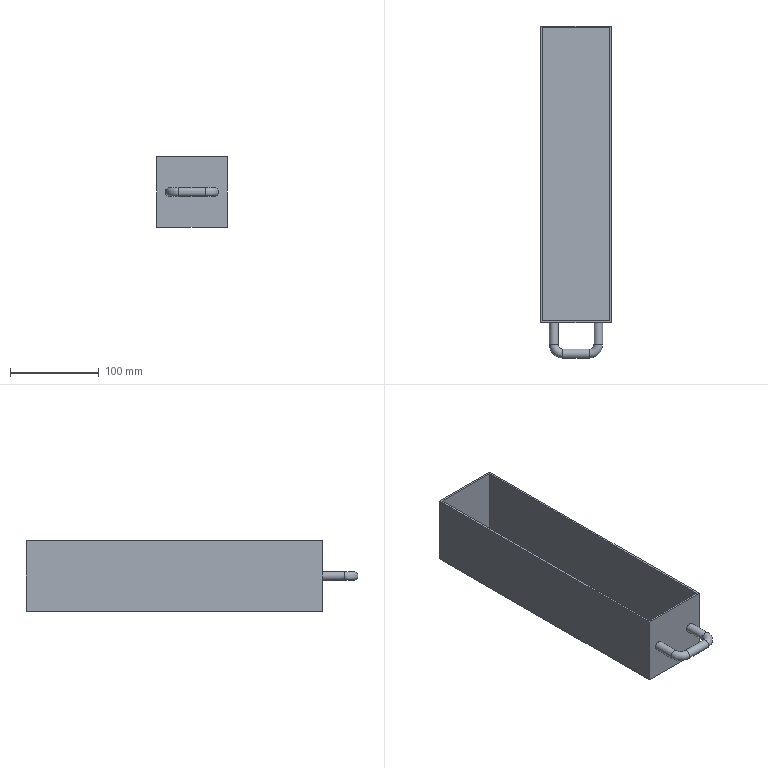Part | NX | features solid 2 | 1 solid | 16 faces | box 80 x 375 x 80 mm | volume 190583 mm3 | plane 11 | cylinder 3 | torus 2 | commonest cylinder face diameters 10 x3
STEP:
#1=CARTESIAN_POINT('',(-100.,-500.,-253.));
#2=VERTEX_POINT('',#1);
#3=CARTESIAN_POINT('',(-100.,-500.,-248.));
#4=DIRECTION('',(0.,1.,0.));
#5=DIRECTION('',(0.,0.,-1.));
#6=AXIS2_PLACEMENT_3D('',#3,#4,#5);
#7=CIRCLE('',#6,5.);
#8=EDGE_CURVE('',#2,#2,#7,.T.);
#9=ORIENTED_EDGE('',*,*,#8,.T.);
#10=EDGE_LOOP('',(#9));
#11=FACE_BOUND('',#10,.T.);
#12=CARTESIAN_POINT('',(-85.,-500.,-208.));
#13=VERTEX_POINT('',#12);
#14=CARTESIAN_POINT('',(-165.,-500.,-208.));
#15=VERTEX_POINT('',#14);
#16=CARTESIAN_POINT('',(-330.,-500.,-208.));
#17=DIRECTION('',(1.,0.,0.));
#18=VECTOR('',#17,1000.);
#19=LINE('',#16,#18);
#20=EDGE_CURVE('',#13,#15,#19,.F.);
#21=ORIENTED_EDGE('',*,*,#20,.T.);
#22=CARTESIAN_POINT('',(-165.,-500.,-288.));
#23=VERTEX_POINT('',#22);
#24=CARTESIAN_POINT('',(-165.,-500.,-208.));
#25=DIRECTION('',(0.,0.,-1.));
#26=VECTOR('',#25,1000.);
#27=LINE('',#24,#26);
#28=EDGE_CURVE('',#23,#15,#27,.F.);
#29=ORIENTED_EDGE('',*,*,#28,.F.);
#30=CARTESIAN_POINT('',(-85.,-500.,-288.));
#31=VERTEX_POINT('',#30);
#32=CARTESIAN_POINT('',(-330.,-500.,-288.));
#33=DIRECTION('',(1.,0.,0.));
#34=VECTOR('',#33,1000.);
#35=LINE('',#32,#34);
#36=EDGE_CURVE('',#31,#23,#35,.F.);
#37=ORIENTED_EDGE('',*,*,#36,.F.);
#38=CARTESIAN_POINT('',(-85.,-500.,-188.));
#39=DIRECTION('',(0.,0.,-1.));
#40=VECTOR('',#39,1000.);
#41=LINE('',#38,#40);
#42=EDGE_CURVE('',#31,#13,#41,.F.);
#43=ORIENTED_EDGE('',*,*,#42,.T.);
#44=EDGE_LOOP('',(#21,#29,#37,#43));
#45=FACE_BOUND('',#44,.T.);
#46=CARTESIAN_POINT('',(-145.,-500.,-248.));
#47=VERTEX_POINT('',#46);
#48=CARTESIAN_POINT('',(-150.,-500.,-248.));
#49=DIRECTION('',(0.,-1.,0.));
#50=DIRECTION('',(1.,0.,0.));
#51=AXIS2_PLACEMENT_3D('',#48,#49,#50);
#52=CIRCLE('',#51,5.);
#53=EDGE_CURVE('',#47,#47,#52,.T.);
#54=ORIENTED_EDGE('',*,*,#53,.F.);
#55=EDGE_LOOP('',(#54));
#56=FACE_BOUND('',#55,.T.);
#57=CARTESIAN_POINT('',(-330.,-500.,-188.));
#58=DIRECTION('',(0.,-1.,0.));
#59=DIRECTION('',(1.,0.,0.));
#60=AXIS2_PLACEMENT_3D('',#57,#58,#59);
#61=PLANE('',#60);
#62=ADVANCED_FACE('',(#11,#45,#56),#61,.T.);
#63=CARTESIAN_POINT('',(-165.,-165.,-208.));
#64=VERTEX_POINT('',#63);
#65=CARTESIAN_POINT('',(-165.,-510.,-208.));
#66=DIRECTION('',(0.,1.,0.));
#67=VECTOR('',#66,1000.);
#68=LINE('',#65,#67);
#69=EDGE_CURVE('',#15,#64,#68,.T.);
#70=ORIENTED_EDGE('',*,*,#69,.T.);
#71=CARTESIAN_POINT('',(-165.,-165.,-288.));
#72=VERTEX_POINT('',#71);
#73=CARTESIAN_POINT('',(-165.,-165.,-208.));
#74=DIRECTION('',(0.,0.,1.));
#75=VECTOR('',#74,1000.);
#76=LINE('',#73,#75);
#77=EDGE_CURVE('',#72,#64,#76,.T.);
#78=ORIENTED_EDGE('',*,*,#77,.F.);
#79=CARTESIAN_POINT('',(-165.,-510.,-288.));
#80=DIRECTION('',(0.,1.,0.));
#81=VECTOR('',#80,1000.);
#82=LINE('',#79,#81);
#83=EDGE_CURVE('',#23,#72,#82,.T.);
#84=ORIENTED_EDGE('',*,*,#83,.F.);
#85=ORIENTED_EDGE('',*,*,#28,.T.);
#86=EDGE_LOOP('',(#70,#78,#84,#85));
#87=FACE_BOUND('',#86,.T.);
#88=CARTESIAN_POINT('',(-165.,-510.,-208.));
#89=DIRECTION('',(1.,0.,0.));
#90=DIRECTION('',(0.,0.,-1.));
#91=AXIS2_PLACEMENT_3D('',#88,#89,#90);
#92=PLANE('',#91);
#93=ADVANCED_FACE('',(#87),#92,.F.);
#94=CARTESIAN_POINT('',(-85.,-165.,-208.));
#95=VERTEX_POINT('',#94);
#96=CARTESIAN_POINT('',(-165.,-165.,-208.));
#97=DIRECTION('',(1.,0.,0.));
#98=VECTOR('',#97,1000.);
#99=LINE('',#96,#98);
#100=EDGE_CURVE('',#64,#95,#99,.T.);
#101=ORIENTED_EDGE('',*,*,#100,.T.);
#102=CARTESIAN_POINT('',(-85.,-165.,-288.));
#103=VERTEX_POINT('',#102);
#104=CARTESIAN_POINT('',(-85.,-165.,-208.));
#105=DIRECTION('',(0.,0.,1.));
#106=VECTOR('',#105,1000.);
#107=LINE('',#104,#106);
#108=EDGE_CURVE('',#103,#95,#107,.T.);
#109=ORIENTED_EDGE('',*,*,#108,.F.);
#110=CARTESIAN_POINT('',(-165.,-165.,-288.));
#111=DIRECTION('',(1.,0.,0.));
#112=VECTOR('',#111,1000.);
#113=LINE('',#110,#112);
#114=EDGE_CURVE('',#72,#103,#113,.T.);
#115=ORIENTED_EDGE('',*,*,#114,.F.);
#116=ORIENTED_EDGE('',*,*,#77,.T.);
#117=EDGE_LOOP('',(#101,#109,#115,#116));
#118=FACE_BOUND('',#117,.T.);
#119=CARTESIAN_POINT('',(-165.,-165.,-208.));
#120=DIRECTION('',(0.,-1.,0.));
#121=DIRECTION('',(0.,0.,-1.));
#122=AXIS2_PLACEMENT_3D('',#119,#120,#121);
#123=PLANE('',#122);
#124=ADVANCED_FACE('',(#118),#123,.F.);
#125=CARTESIAN_POINT('',(-85.,-165.,-208.));
#126=DIRECTION('',(0.,-1.,0.));
#127=VECTOR('',#126,1000.);
#128=LINE('',#125,#127);
#129=EDGE_CURVE('',#95,#13,#128,.T.);
#130=ORIENTED_EDGE('',*,*,#129,.T.);
#131=ORIENTED_EDGE('',*,*,#42,.F.);
#132=CARTESIAN_POINT('',(-85.,-165.,-288.));
#133=DIRECTION('',(0.,-1.,0.));
#134=VECTOR('',#133,1000.);
#135=LINE('',#132,#134);
#136=EDGE_CURVE('',#103,#31,#135,.T.);
#137=ORIENTED_EDGE('',*,*,#136,.F.);
#138=ORIENTED_EDGE('',*,*,#108,.T.);
#139=EDGE_LOOP('',(#130,#131,#137,#138));
#140=FACE_BOUND('',#139,.T.);
#141=CARTESIAN_POINT('',(-85.,-165.,-208.));
#142=DIRECTION('',(-1.,0.,0.));
#143=DIRECTION('',(0.,0.,1.));
#144=AXIS2_PLACEMENT_3D('',#141,#142,#143);
#145=PLANE('',#144);
#146=ADVANCED_FACE('',(#140),#145,.F.);
#147=ORIENTED_EDGE('',*,*,#36,.T.);
#148=ORIENTED_EDGE('',*,*,#83,.T.);
#149=ORIENTED_EDGE('',*,*,#114,.T.);
#150=ORIENTED_EDGE('',*,*,#136,.T.);
#151=EDGE_LOOP('',(#147,#148,#149,#150));
#152=FACE_BOUND('',#151,.T.);
#153=CARTESIAN_POINT('',(-165.,-510.,-288.));
#154=DIRECTION('',(0.,0.,-1.));
#155=DIRECTION('',(-1.,0.,0.));
#156=AXIS2_PLACEMENT_3D('',#153,#154,#155);
#157=PLANE('',#156);
#158=ADVANCED_FACE('',(#152),#157,.T.);
#159=CARTESIAN_POINT('',(-87.,-167.,-208.));
#160=VERTEX_POINT('',#159);
#161=CARTESIAN_POINT('',(-87.,-498.,-208.));
#162=VERTEX_POINT('',#161);
#163=CARTESIAN_POINT('',(-87.,-165.,-208.));
#164=DIRECTION('',(0.,-1.,0.));
#165=VECTOR('',#164,1000.);
#166=LINE('',#163,#165);
#167=EDGE_CURVE('',#160,#162,#166,.T.);
#168=ORIENTED_EDGE('',*,*,#167,.T.);
#169=CARTESIAN_POINT('',(-163.,-498.,-208.));
#170=VERTEX_POINT('',#169);
#171=CARTESIAN_POINT('',(-330.,-498.,-208.));
#172=DIRECTION('',(1.,0.,0.));
#173=VECTOR('',#172,1000.);
#174=LINE('',#171,#173);
#175=EDGE_CURVE('',#162,#170,#174,.F.);
#176=ORIENTED_EDGE('',*,*,#175,.T.);
#177=CARTESIAN_POINT('',(-163.,-167.,-208.));
#178=VERTEX_POINT('',#177);
#179=CARTESIAN_POINT('',(-163.,-510.,-208.));
#180=DIRECTION('',(0.,1.,0.));
#181=VECTOR('',#180,1000.);
#182=LINE('',#179,#181);
#183=EDGE_CURVE('',#170,#178,#182,.T.);
#184=ORIENTED_EDGE('',*,*,#183,.T.);
#185=CARTESIAN_POINT('',(-165.,-167.,-208.));
#186=DIRECTION('',(1.,0.,0.));
#187=VECTOR('',#186,1000.);
#188=LINE('',#185,#187);
#189=EDGE_CURVE('',#178,#160,#188,.T.);
#190=ORIENTED_EDGE('',*,*,#189,.T.);
#191=EDGE_LOOP('',(#168,#176,#184,#190));
#192=FACE_BOUND('',#191,.T.);
#193=ORIENTED_EDGE('',*,*,#20,.F.);
#194=ORIENTED_EDGE('',*,*,#129,.F.);
#195=ORIENTED_EDGE('',*,*,#100,.F.);
#196=ORIENTED_EDGE('',*,*,#69,.F.);
#197=EDGE_LOOP('',(#193,#194,#195,#196));
#198=FACE_BOUND('',#197,.T.);
#199=CARTESIAN_POINT('',(-165.,-510.,-208.));
#200=DIRECTION('',(0.,0.,-1.));
#201=DIRECTION('',(-1.,0.,0.));
#202=AXIS2_PLACEMENT_3D('',#199,#200,#201);
#203=PLANE('',#202);
#204=ADVANCED_FACE('',(#192,#198),#203,.F.);
#205=ORIENTED_EDGE('',*,*,#175,.F.);
#206=CARTESIAN_POINT('',(-87.,-498.,-286.));
#207=VERTEX_POINT('',#206);
#208=CARTESIAN_POINT('',(-87.,-498.,-188.));
#209=DIRECTION('',(0.,0.,-1.));
#210=VECTOR('',#209,1000.);
#211=LINE('',#208,#210);
#212=EDGE_CURVE('',#207,#162,#211,.F.);
#213=ORIENTED_EDGE('',*,*,#212,.F.);
#214=CARTESIAN_POINT('',(-163.,-498.,-286.));
#215=VERTEX_POINT('',#214);
#216=CARTESIAN_POINT('',(-330.,-498.,-286.));
#217=DIRECTION('',(1.,0.,0.));
#218=VECTOR('',#217,1000.);
#219=LINE('',#216,#218);
#220=EDGE_CURVE('',#207,#215,#219,.F.);
#221=ORIENTED_EDGE('',*,*,#220,.T.);
#222=CARTESIAN_POINT('',(-163.,-498.,-208.));
#223=DIRECTION('',(0.,0.,-1.));
#224=VECTOR('',#223,1000.);
#225=LINE('',#222,#224);
#226=EDGE_CURVE('',#215,#170,#225,.F.);
#227=ORIENTED_EDGE('',*,*,#226,.T.);
#228=EDGE_LOOP('',(#205,#213,#221,#227));
#229=FACE_BOUND('',#228,.T.);
#230=CARTESIAN_POINT('',(-330.,-498.,-188.));
#231=DIRECTION('',(0.,-1.,0.));
#232=DIRECTION('',(1.,0.,0.));
#233=AXIS2_PLACEMENT_3D('',#230,#231,#232);
#234=PLANE('',#233);
#235=ADVANCED_FACE('',(#229),#234,.F.);
#236=ORIENTED_EDGE('',*,*,#183,.F.);
#237=ORIENTED_EDGE('',*,*,#226,.F.);
#238=CARTESIAN_POINT('',(-163.,-167.,-286.));
#239=VERTEX_POINT('',#238);
#240=CARTESIAN_POINT('',(-163.,-510.,-286.));
#241=DIRECTION('',(0.,1.,0.));
#242=VECTOR('',#241,1000.);
#243=LINE('',#240,#242);
#244=EDGE_CURVE('',#215,#239,#243,.T.);
#245=ORIENTED_EDGE('',*,*,#244,.T.);
#246=CARTESIAN_POINT('',(-163.,-167.,-208.));
#247=DIRECTION('',(0.,0.,1.));
#248=VECTOR('',#247,1000.);
#249=LINE('',#246,#248);
#250=EDGE_CURVE('',#239,#178,#249,.T.);
#251=ORIENTED_EDGE('',*,*,#250,.T.);
#252=EDGE_LOOP('',(#236,#237,#245,#251));
#253=FACE_BOUND('',#252,.T.);
#254=CARTESIAN_POINT('',(-163.,-510.,-208.));
#255=DIRECTION('',(1.,0.,0.));
#256=DIRECTION('',(0.,0.,-1.));
#257=AXIS2_PLACEMENT_3D('',#254,#255,#256);
#258=PLANE('',#257);
#259=ADVANCED_FACE('',(#253),#258,.T.);
#260=ORIENTED_EDGE('',*,*,#189,.F.);
#261=ORIENTED_EDGE('',*,*,#250,.F.);
#262=CARTESIAN_POINT('',(-87.,-167.,-286.));
#263=VERTEX_POINT('',#262);
#264=CARTESIAN_POINT('',(-165.,-167.,-286.));
#265=DIRECTION('',(1.,0.,0.));
#266=VECTOR('',#265,1000.);
#267=LINE('',#264,#266);
#268=EDGE_CURVE('',#239,#263,#267,.T.);
#269=ORIENTED_EDGE('',*,*,#268,.T.);
#270=CARTESIAN_POINT('',(-87.,-167.,-208.));
#271=DIRECTION('',(0.,0.,1.));
#272=VECTOR('',#271,1000.);
#273=LINE('',#270,#272);
#274=EDGE_CURVE('',#263,#160,#273,.T.);
#275=ORIENTED_EDGE('',*,*,#274,.T.);
#276=EDGE_LOOP('',(#260,#261,#269,#275));
#277=FACE_BOUND('',#276,.T.);
#278=CARTESIAN_POINT('',(-165.,-167.,-208.));
#279=DIRECTION('',(0.,-1.,0.));
#280=DIRECTION('',(0.,0.,-1.));
#281=AXIS2_PLACEMENT_3D('',#278,#279,#280);
#282=PLANE('',#281);
#283=ADVANCED_FACE('',(#277),#282,.T.);
#284=ORIENTED_EDGE('',*,*,#167,.F.);
#285=ORIENTED_EDGE('',*,*,#274,.F.);
#286=CARTESIAN_POINT('',(-87.,-165.,-286.));
#287=DIRECTION('',(0.,-1.,0.));
#288=VECTOR('',#287,1000.);
#289=LINE('',#286,#288);
#290=EDGE_CURVE('',#263,#207,#289,.T.);
#291=ORIENTED_EDGE('',*,*,#290,.T.);
#292=ORIENTED_EDGE('',*,*,#212,.T.);
#293=EDGE_LOOP('',(#284,#285,#291,#292));
#294=FACE_BOUND('',#293,.T.);
#295=CARTESIAN_POINT('',(-87.,-165.,-208.));
#296=DIRECTION('',(-1.,0.,0.));
#297=DIRECTION('',(0.,0.,1.));
#298=AXIS2_PLACEMENT_3D('',#295,#296,#297);
#299=PLANE('',#298);
#300=ADVANCED_FACE('',(#294),#299,.T.);
#301=ORIENTED_EDGE('',*,*,#220,.F.);
#302=ORIENTED_EDGE('',*,*,#290,.F.);
#303=ORIENTED_EDGE('',*,*,#268,.F.);
#304=ORIENTED_EDGE('',*,*,#244,.F.);
#305=EDGE_LOOP('',(#301,#302,#303,#304));
#306=FACE_BOUND('',#305,.T.);
#307=CARTESIAN_POINT('',(-165.,-510.,-286.));
#308=DIRECTION('',(0.,0.,-1.));
#309=DIRECTION('',(-1.,0.,0.));
#310=AXIS2_PLACEMENT_3D('',#307,#308,#309);
#311=PLANE('',#310);
#312=ADVANCED_FACE('',(#306),#311,.F.);
#313=CARTESIAN_POINT('',(-100.,-525.,-253.));
#314=VERTEX_POINT('',#313);
#315=CARTESIAN_POINT('',(-100.,-525.,-248.));
#316=DIRECTION('',(0.,1.,0.));
#317=DIRECTION('',(0.,0.,-1.));
#318=AXIS2_PLACEMENT_3D('',#315,#316,#317);
#319=CIRCLE('',#318,5.);
#320=EDGE_CURVE('',#314,#314,#319,.T.);
#321=ORIENTED_EDGE('',*,*,#320,.T.);
#322=EDGE_LOOP('',(#321));
#323=FACE_BOUND('',#322,.T.);
#324=ORIENTED_EDGE('',*,*,#8,.F.);
#325=EDGE_LOOP('',(#324));
#326=FACE_BOUND('',#325,.T.);
#327=CARTESIAN_POINT('',(-100.,-525.,-248.));
#328=DIRECTION('',(0.,1.,0.));
#329=DIRECTION('',(0.,0.,1.));
#330=AXIS2_PLACEMENT_3D('',#327,#328,#329);
#331=CYLINDRICAL_SURFACE('',#330,5.);
#332=ADVANCED_FACE('',(#323,#326),#331,.T.);
#333=CARTESIAN_POINT('',(-110.,-535.,-253.));
#334=VERTEX_POINT('',#333);
#335=CARTESIAN_POINT('',(-110.,-535.,-248.));
#336=DIRECTION('',(1.,0.,0.));
#337=DIRECTION('',(0.,0.,-1.));
#338=AXIS2_PLACEMENT_3D('',#335,#336,#337);
#339=CIRCLE('',#338,5.);
#340=EDGE_CURVE('',#334,#334,#339,.T.);
#341=ORIENTED_EDGE('',*,*,#340,.T.);
#342=EDGE_LOOP('',(#341));
#343=FACE_BOUND('',#342,.T.);
#344=ORIENTED_EDGE('',*,*,#320,.F.);
#345=EDGE_LOOP('',(#344));
#346=FACE_BOUND('',#345,.T.);
#347=CARTESIAN_POINT('',(-110.,-525.,-248.));
#348=DIRECTION('',(0.,0.,1.));
#349=DIRECTION('',(1.,0.,0.));
#350=AXIS2_PLACEMENT_3D('',#347,#348,#349);
#351=TOROIDAL_SURFACE('',#350,10.,5.);
#352=ADVANCED_FACE('',(#343,#346),#351,.T.);
#353=CARTESIAN_POINT('',(-140.,-535.,-253.));
#354=VERTEX_POINT('',#353);
#355=CARTESIAN_POINT('',(-140.,-535.,-248.));
#356=DIRECTION('',(1.,0.,0.));
#357=DIRECTION('',(0.,0.,-1.));
#358=AXIS2_PLACEMENT_3D('',#355,#356,#357);
#359=CIRCLE('',#358,5.);
#360=EDGE_CURVE('',#354,#354,#359,.T.);
#361=ORIENTED_EDGE('',*,*,#360,.T.);
#362=EDGE_LOOP('',(#361));
#363=FACE_BOUND('',#362,.T.);
#364=ORIENTED_EDGE('',*,*,#340,.F.);
#365=EDGE_LOOP('',(#364));
#366=FACE_BOUND('',#365,.T.);
#367=CARTESIAN_POINT('',(-140.,-535.,-248.));
#368=DIRECTION('',(1.,0.,0.));
#369=DIRECTION('',(0.,0.,-1.));
#370=AXIS2_PLACEMENT_3D('',#367,#368,#369);
#371=CYLINDRICAL_SURFACE('',#370,5.);
#372=ADVANCED_FACE('',(#363,#366),#371,.T.);
#373=CARTESIAN_POINT('',(-150.,-525.,-253.));
#374=VERTEX_POINT('',#373);
#375=CARTESIAN_POINT('',(-150.,-525.,-248.));
#376=DIRECTION('',(0.,-1.,0.));
#377=DIRECTION('',(0.,0.,-1.));
#378=AXIS2_PLACEMENT_3D('',#375,#376,#377);
#379=CIRCLE('',#378,5.);
#380=EDGE_CURVE('',#374,#374,#379,.T.);
#381=ORIENTED_EDGE('',*,*,#380,.T.);
#382=EDGE_LOOP('',(#381));
#383=FACE_BOUND('',#382,.T.);
#384=ORIENTED_EDGE('',*,*,#360,.F.);
#385=EDGE_LOOP('',(#384));
#386=FACE_BOUND('',#385,.T.);
#387=CARTESIAN_POINT('',(-140.,-525.,-248.));
#388=DIRECTION('',(0.,0.,1.));
#389=DIRECTION('',(1.,0.,0.));
#390=AXIS2_PLACEMENT_3D('',#387,#388,#389);
#391=TOROIDAL_SURFACE('',#390,10.,5.);
#392=ADVANCED_FACE('',(#383,#386),#391,.T.);
#393=ORIENTED_EDGE('',*,*,#380,.F.);
#394=EDGE_LOOP('',(#393));
#395=FACE_BOUND('',#394,.T.);
#396=ORIENTED_EDGE('',*,*,#53,.T.);
#397=EDGE_LOOP('',(#396));
#398=FACE_BOUND('',#397,.T.);
#399=CARTESIAN_POINT('',(-150.,-525.,-248.));
#400=DIRECTION('',(0.,1.,0.));
#401=DIRECTION('',(0.,0.,1.));
#402=AXIS2_PLACEMENT_3D('',#399,#400,#401);
#403=CYLINDRICAL_SURFACE('',#402,5.);
#404=ADVANCED_FACE('',(#395,#398),#403,.T.);
#405=CLOSED_SHELL('',(#62,#93,#124,#146,#158,#204,#235,#259,#283,#300,#312,#332,#352,#372,#392,#404));
#406=MANIFOLD_SOLID_BREP('',#405);
#407=(LENGTH_UNIT()NAMED_UNIT(*)SI_UNIT(.MILLI.,.METRE.));
#408=UNCERTAINTY_MEASURE_WITH_UNIT(LENGTH_MEASURE(0.00001),#407,'','');
#409=(NAMED_UNIT(*)PLANE_ANGLE_UNIT()SI_UNIT($,.RADIAN.));
#410=(NAMED_UNIT(*)SI_UNIT($,.STERADIAN.)SOLID_ANGLE_UNIT());
#411=(GEOMETRIC_REPRESENTATION_CONTEXT(3)GLOBAL_UNCERTAINTY_ASSIGNED_CONTEXT((#408))GLOBAL_UNIT_ASSIGNED_CONTEXT((#407,#409,#410))REPRESENTATION_CONTEXT('',''));
#412=ADVANCED_BREP_SHAPE_REPRESENTATION('',(#406),#411);